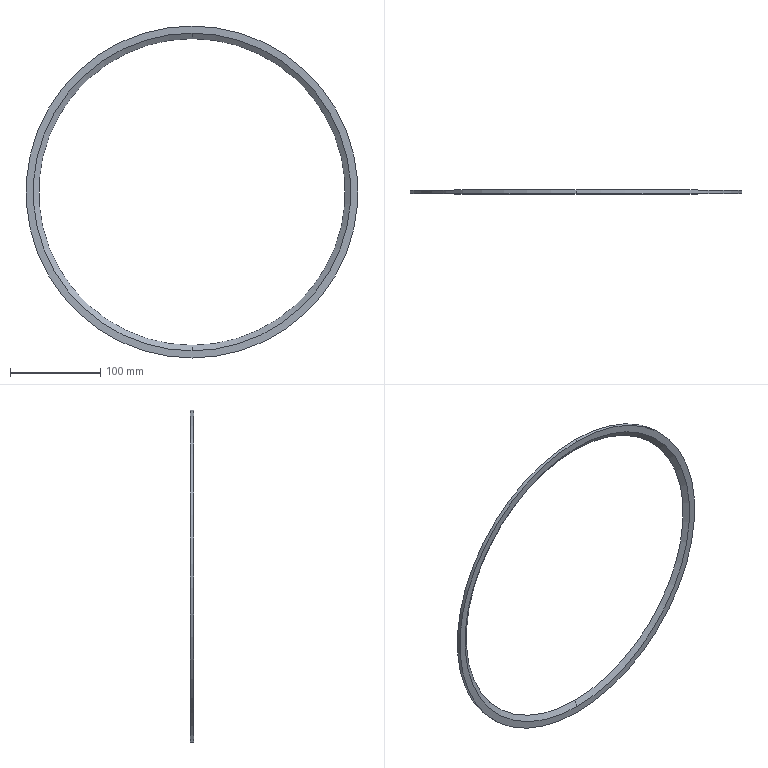Part | SolidWorks | features Revolution 1 | 1 solid | 6 faces | box 368 x 4 x 368 mm | volume 49310 mm3 | cylinder 2 | cone 2 | plane 2 | commonest cylinder face diameters 368 x2
STEP:
#1=CARTESIAN_POINT('',(0.,4.,-184.));
#2=VERTEX_POINT('',#1);
#3=CARTESIAN_POINT('',(0.,4.,184.));
#4=VERTEX_POINT('',#3);
#5=CARTESIAN_POINT('',(0.,4.,0.));
#6=DIRECTION('',(0.,-1.,0.));
#7=DIRECTION('',(0.,0.,-1.));
#8=AXIS2_PLACEMENT_3D('',#5,#6,#7);
#9=CIRCLE('',#8,184.);
#10=EDGE_CURVE('',#2,#4,#9,.T.);
#11=ORIENTED_EDGE('',*,*,#10,.T.);
#12=CARTESIAN_POINT('',(0.,0.,184.));
#13=VERTEX_POINT('',#12);
#14=CARTESIAN_POINT('',(0.,23.758,184.));
#15=DIRECTION('',(0.,-1.,0.));
#16=VECTOR('',#15,1000.);
#17=LINE('',#14,#16);
#18=EDGE_CURVE('',#4,#13,#17,.T.);
#19=ORIENTED_EDGE('',*,*,#18,.T.);
#20=CARTESIAN_POINT('',(0.,0.,-184.));
#21=VERTEX_POINT('',#20);
#22=CARTESIAN_POINT('',(0.,0.,0.));
#23=DIRECTION('',(0.,-1.,0.));
#24=DIRECTION('',(0.,0.,-1.));
#25=AXIS2_PLACEMENT_3D('',#22,#23,#24);
#26=CIRCLE('',#25,184.);
#27=EDGE_CURVE('',#21,#13,#26,.T.);
#28=ORIENTED_EDGE('',*,*,#27,.F.);
#29=CARTESIAN_POINT('',(0.,23.758,-184.));
#30=DIRECTION('',(0.,-1.,0.));
#31=VECTOR('',#30,1000.);
#32=LINE('',#29,#31);
#33=EDGE_CURVE('',#2,#21,#32,.T.);
#34=ORIENTED_EDGE('',*,*,#33,.F.);
#35=EDGE_LOOP('',(#11,#19,#28,#34));
#36=FACE_OUTER_BOUND('',#35,.T.);
#37=CARTESIAN_POINT('',(0.,23.758,0.));
#38=DIRECTION('',(0.,-1.,0.));
#39=DIRECTION('',(0.,0.,-1.));
#40=AXIS2_PLACEMENT_3D('',#37,#38,#39);
#41=CYLINDRICAL_SURFACE('',#40,184.);
#42=ADVANCED_FACE('',(#36),#41,.T.);
#43=CARTESIAN_POINT('',(0.,4.,170.));
#44=VERTEX_POINT('',#43);
#45=CARTESIAN_POINT('',(0.,4.,-170.));
#46=VERTEX_POINT('',#45);
#47=CARTESIAN_POINT('',(0.,4.,0.));
#48=DIRECTION('',(0.,-1.,0.));
#49=DIRECTION('',(0.,0.,-1.));
#50=AXIS2_PLACEMENT_3D('',#47,#48,#49);
#51=CIRCLE('',#50,170.);
#52=EDGE_CURVE('',#44,#46,#51,.T.);
#53=ORIENTED_EDGE('',*,*,#52,.F.);
#54=CARTESIAN_POINT('',(0.,0.,176.));
#55=VERTEX_POINT('',#54);
#56=CARTESIAN_POINT('',(0.,0.,176.));
#57=DIRECTION('',(0.,-0.5547,0.8321));
#58=VECTOR('',#57,1000.);
#59=LINE('',#56,#58);
#60=EDGE_CURVE('',#44,#55,#59,.T.);
#61=ORIENTED_EDGE('',*,*,#60,.T.);
#62=CARTESIAN_POINT('',(0.,0.,-176.));
#63=VERTEX_POINT('',#62);
#64=CARTESIAN_POINT('',(0.,0.,0.));
#65=DIRECTION('',(0.,-1.,0.));
#66=DIRECTION('',(0.,0.,-1.));
#67=AXIS2_PLACEMENT_3D('',#64,#65,#66);
#68=CIRCLE('',#67,176.);
#69=EDGE_CURVE('',#55,#63,#68,.T.);
#70=ORIENTED_EDGE('',*,*,#69,.T.);
#71=CARTESIAN_POINT('',(0.,0.,-176.));
#72=DIRECTION('',(0.,-0.5547,-0.8321));
#73=VECTOR('',#72,1000.);
#74=LINE('',#71,#73);
#75=EDGE_CURVE('',#46,#63,#74,.T.);
#76=ORIENTED_EDGE('',*,*,#75,.F.);
#77=EDGE_LOOP('',(#53,#61,#70,#76));
#78=FACE_OUTER_BOUND('',#77,.T.);
#79=CARTESIAN_POINT('',(0.,0.,0.));
#80=DIRECTION('',(0.,-1.,0.));
#81=DIRECTION('',(0.,0.,-1.));
#82=AXIS2_PLACEMENT_3D('',#79,#80,#81);
#83=CONICAL_SURFACE('',#82,176.,0.9828);
#84=ADVANCED_FACE('',(#78),#83,.F.);
#85=ORIENTED_EDGE('',*,*,#60,.F.);
#86=CARTESIAN_POINT('',(0.,4.,0.));
#87=DIRECTION('',(0.,-1.,0.));
#88=DIRECTION('',(0.,0.,-1.));
#89=AXIS2_PLACEMENT_3D('',#86,#87,#88);
#90=CIRCLE('',#89,170.);
#91=EDGE_CURVE('',#46,#44,#90,.T.);
#92=ORIENTED_EDGE('',*,*,#91,.F.);
#93=ORIENTED_EDGE('',*,*,#75,.T.);
#94=CARTESIAN_POINT('',(0.,0.,0.));
#95=DIRECTION('',(0.,-1.,0.));
#96=DIRECTION('',(0.,0.,-1.));
#97=AXIS2_PLACEMENT_3D('',#94,#95,#96);
#98=CIRCLE('',#97,176.);
#99=EDGE_CURVE('',#63,#55,#98,.T.);
#100=ORIENTED_EDGE('',*,*,#99,.T.);
#101=EDGE_LOOP('',(#85,#92,#93,#100));
#102=FACE_OUTER_BOUND('',#101,.T.);
#103=CARTESIAN_POINT('',(0.,0.,0.));
#104=DIRECTION('',(0.,-1.,0.));
#105=DIRECTION('',(0.,0.,-1.));
#106=AXIS2_PLACEMENT_3D('',#103,#104,#105);
#107=CONICAL_SURFACE('',#106,176.,0.9828);
#108=ADVANCED_FACE('',(#102),#107,.F.);
#109=ORIENTED_EDGE('',*,*,#99,.F.);
#110=ORIENTED_EDGE('',*,*,#69,.F.);
#111=EDGE_LOOP('',(#109,#110));
#112=FACE_BOUND('',#111,.T.);
#113=ORIENTED_EDGE('',*,*,#27,.T.);
#114=CARTESIAN_POINT('',(0.,0.,0.));
#115=DIRECTION('',(0.,-1.,0.));
#116=DIRECTION('',(0.,0.,-1.));
#117=AXIS2_PLACEMENT_3D('',#114,#115,#116);
#118=CIRCLE('',#117,184.);
#119=EDGE_CURVE('',#13,#21,#118,.T.);
#120=ORIENTED_EDGE('',*,*,#119,.T.);
#121=EDGE_LOOP('',(#113,#120));
#122=FACE_OUTER_BOUND('',#121,.T.);
#123=CARTESIAN_POINT('',(-184.,0.,0.));
#124=DIRECTION('',(0.,1.,0.));
#125=DIRECTION('',(0.,0.,1.));
#126=AXIS2_PLACEMENT_3D('',#123,#124,#125);
#127=PLANE('',#126);
#128=ADVANCED_FACE('',(#112,#122),#127,.F.);
#129=ORIENTED_EDGE('',*,*,#18,.F.);
#130=CARTESIAN_POINT('',(0.,4.,0.));
#131=DIRECTION('',(0.,-1.,0.));
#132=DIRECTION('',(0.,0.,-1.));
#133=AXIS2_PLACEMENT_3D('',#130,#131,#132);
#134=CIRCLE('',#133,184.);
#135=EDGE_CURVE('',#4,#2,#134,.T.);
#136=ORIENTED_EDGE('',*,*,#135,.T.);
#137=ORIENTED_EDGE('',*,*,#33,.T.);
#138=ORIENTED_EDGE('',*,*,#119,.F.);
#139=EDGE_LOOP('',(#129,#136,#137,#138));
#140=FACE_OUTER_BOUND('',#139,.T.);
#141=CARTESIAN_POINT('',(0.,23.758,0.));
#142=DIRECTION('',(0.,-1.,0.));
#143=DIRECTION('',(0.,0.,-1.));
#144=AXIS2_PLACEMENT_3D('',#141,#142,#143);
#145=CYLINDRICAL_SURFACE('',#144,184.);
#146=ADVANCED_FACE('',(#140),#145,.T.);
#147=ORIENTED_EDGE('',*,*,#10,.F.);
#148=ORIENTED_EDGE('',*,*,#135,.F.);
#149=EDGE_LOOP('',(#147,#148));
#150=FACE_OUTER_BOUND('',#149,.T.);
#151=ORIENTED_EDGE('',*,*,#91,.T.);
#152=ORIENTED_EDGE('',*,*,#52,.T.);
#153=EDGE_LOOP('',(#151,#152));
#154=FACE_BOUND('',#153,.T.);
#155=CARTESIAN_POINT('',(-170.,4.,0.));
#156=DIRECTION('',(0.,-1.,0.));
#157=DIRECTION('',(0.,0.,-1.));
#158=AXIS2_PLACEMENT_3D('',#155,#156,#157);
#159=PLANE('',#158);
#160=ADVANCED_FACE('',(#150,#154),#159,.F.);
#161=CLOSED_SHELL('',(#42,#84,#108,#128,#146,#160));
#162=MANIFOLD_SOLID_BREP('',#161);
#163=CARTESIAN_POINT('',(0.,0.,0.));
#164=DIRECTION('',(0.,0.,1.));
#165=DIRECTION('',(1.,0.,0.));
#166=AXIS2_PLACEMENT_3D('',#163,#164,#165);
#167=(LENGTH_UNIT()NAMED_UNIT(*)SI_UNIT(.MILLI.,.METRE.));
#168=UNCERTAINTY_MEASURE_WITH_UNIT(LENGTH_MEASURE(0.00001),#167,'','');
#169=(NAMED_UNIT(*)PLANE_ANGLE_UNIT()SI_UNIT($,.RADIAN.));
#170=(NAMED_UNIT(*)SI_UNIT($,.STERADIAN.)SOLID_ANGLE_UNIT());
#171=(GEOMETRIC_REPRESENTATION_CONTEXT(3)GLOBAL_UNCERTAINTY_ASSIGNED_CONTEXT((#168))GLOBAL_UNIT_ASSIGNED_CONTEXT((#167,#169,#170))REPRESENTATION_CONTEXT('',''));
#172=ADVANCED_BREP_SHAPE_REPRESENTATION('',(#162,#166),#171);